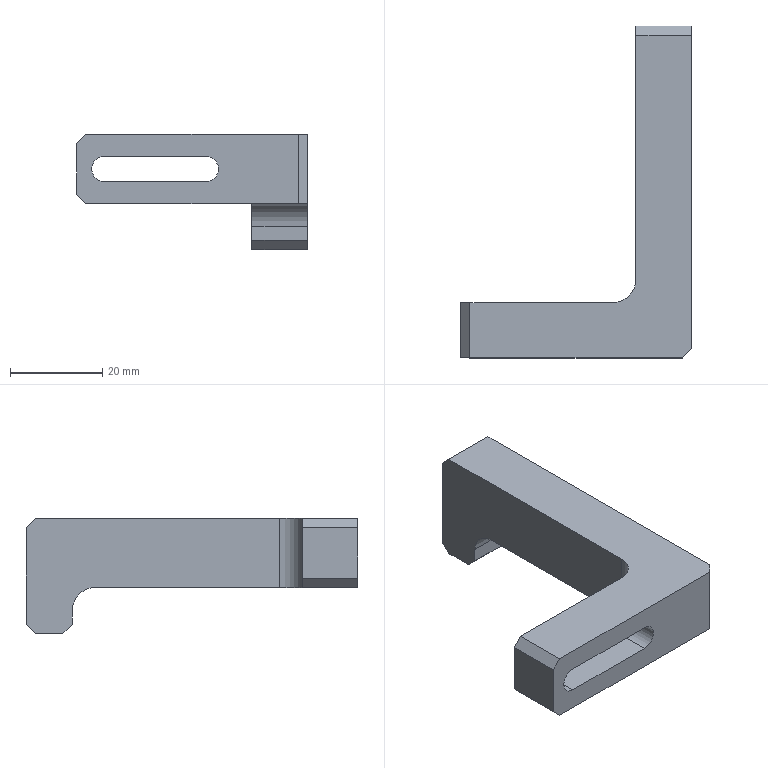NC program | NX | posted with a generic post | part box 50 x 72 x 25 mm
Lines 1 to 975 of 3150:
N10 G17 G21 G94 G90
(ZLEVEL_PROFILE_COPY_COPY_1 , TOOL : D3)
N12 T16 M6
N14 G54
N16 G17 G0 G90 X3.75 Y-1.724 B0. C0. S9500 M3
N18 G43 Z30. H16
N20 Z0.6
N22 G94 G1 Y-3.158 Z0.525 F1000.
N24 X3.81 Y-3.413 Z0.511
N26 X3.95 Y-3.697 Z0.495
N28 X4.25 Y-4.012 Z0.472
N30 X4.639 Y-4.207 Z0.449
N32 X5.071 Y-4.258 Z0.426
N34 X5.495 Y-4.159 Z0.403
N36 X5.86 Y-3.921 Z0.38
N38 X6.062 Y-3.677 Z0.364
N40 X6.185 Y-3.428 Z0.349
N42 X6.25 Y-3.158 Z0.335
N44 Y8. Z-0.25
N46 Y19. F1200.
N48 G3 X5. Y20.25 R1.25
N50 X3.75 Y19. R1.25
N52 G1 Y-3.
N54 G3 X5. Y-4.25 R1.25
N56 X6.25 Y-3. R1.25
N58 G1 Y8.
N60 Y17.625 Z-0.296
N62 X6.246 Y19. Z-0.303
N64 X6.232 Y19.165 Z-0.304
N66 X6.214 Y19.262
N68 X6.174 Y19.415 Z-0.305
N70 X6.132 Y19.513 Z-0.306
N72 X6.048 Y19.665
N74 X5.999 Y19.742 Z-0.307
N76 X5.903 Y19.852 Z-0.308
N78 X5.82 Y19.936
N80 X5.71 Y20.022 Z-0.309
N82 X5.603 Y20.086
N84 X5.44 Y20.161 Z-0.31
N86 X5.339 Y20.197 Z-0.311
N88 X5.186 Y20.227 Z-0.312
N90 X5.056 Y20.241
N92 X4.951 Y20.242 Z-0.313
N94 X4.899
N96 X4.856 Y20.235
N98 X4.77 Y20.221 Z-0.314
N100 X4.586 Y20.17 Z-0.315
N102 X4.495 Y20.14
N104 X4.37 Y20.07 Z-0.316
N106 X4.25 Y19.991
N108 X4.127 Y19.886 Z-0.317
N110 X4.044 Y19.793 Z-0.318
N112 X3.944 Y19.653 Z-0.319
N114 X3.888 Y19.553
N116 X3.843 Y19.454 Z-0.32
N118 X3.821 Y19.404
N120 X3.811 Y19.364
N122 X3.791 Y19.284 Z-0.321
N124 X3.766 Y19.143
N126 X3.754 Y19. Z-0.322
N128 X3.75 Y17.625 Z-0.329
N130 Y-1.625 Z-0.421
N132 X3.754 Y-3. Z-0.428
N134 X3.769 Y-3.18 Z-0.429
N136 X3.79 Y-3.283
N138 X3.843 Y-3.454 Z-0.43
N140 X3.887 Y-3.552 Z-0.431
N142 X3.98 Y-3.71 Z-0.432
N144 X4.057 Y-3.808
N146 X4.185 Y-3.938 Z-0.433
N148 X4.284 Y-4.016 Z-0.434
N150 X4.44 Y-4.11 Z-0.435
N152 X4.556 Y-4.16
N154 X4.73 Y-4.213 Z-0.436
N156 X4.855 Y-4.234 Z-0.437
N158 X5.037 Y-4.242 Z-0.438
N160 X5.163 Y-4.232
N162 X5.341 Y-4.195 Z-0.439
N164 X5.461 Y-4.154 Z-0.44
N166 X5.625 Y-4.074 Z-0.441
N168 X5.731 Y-4.005
N170 X5.868 Y-3.889 Z-0.442
N172 X5.955 Y-3.794 Z-0.443
N174 X6.053 Y-3.659 Z-0.444
N176 X6.112 Y-3.554
N178 X6.155 Y-3.458 Z-0.445
N180 X6.177 Y-3.41
N182 X6.187 Y-3.368
N184 X6.209 Y-3.285 Z-0.446
N186 X6.226 Y-3.214
N188 X6.242 Y-3.144
N190 X6.248 Y-3.072 Z-0.447
N192 X6.25 Y-3.
N194 Y8. Z-0.5
N196 Y17.625 Z-0.546
N198 X6.246 Y19. Z-0.553
N200 X6.232 Y19.165 Z-0.554
N202 X6.214 Y19.262
N204 X6.174 Y19.415 Z-0.555
N206 X6.132 Y19.513 Z-0.556
N208 X6.048 Y19.665
N210 X5.999 Y19.742 Z-0.557
N212 X5.903 Y19.852 Z-0.558
N214 X5.82 Y19.936
N216 X5.71 Y20.022 Z-0.559
N218 X5.603 Y20.086
N220 X5.44 Y20.161 Z-0.56
N222 X5.339 Y20.197 Z-0.561
N224 X5.187 Y20.227 Z-0.562
N226 X5.056 Y20.241
N228 X4.951 Y20.242 Z-0.563
N230 X4.899
N232 X4.856 Y20.235
N234 X4.77 Y20.221 Z-0.564
N236 X4.586 Y20.17 Z-0.565
N238 X4.495 Y20.14
N240 X4.37 Y20.07 Z-0.566
N242 X4.25 Y19.991
N244 X4.127 Y19.886 Z-0.567
N246 X4.044 Y19.793 Z-0.568
N248 X3.944 Y19.653 Z-0.569
N250 X3.888 Y19.553
N252 X3.843 Y19.454 Z-0.57
N254 X3.821 Y19.404
N256 X3.811 Y19.364
N258 X3.791 Y19.284 Z-0.571
N260 X3.766 Y19.143
N262 X3.754 Y19. Z-0.572
N264 X3.75 Y17.625 Z-0.579
N266 Y-1.625 Z-0.671
N268 X3.754 Y-3. Z-0.678
N270 X3.769 Y-3.18 Z-0.679
N272 X3.79 Y-3.283
N274 X3.843 Y-3.454 Z-0.68
N276 X3.887 Y-3.552 Z-0.681
N278 X3.98 Y-3.71 Z-0.682
N280 X4.057 Y-3.808
N282 X4.185 Y-3.938 Z-0.683
N284 X4.284 Y-4.016 Z-0.684
N286 X4.44 Y-4.11 Z-0.685
N288 X4.556 Y-4.16
N290 X4.73 Y-4.213 Z-0.686
N292 X4.855 Y-4.234 Z-0.687
N294 X5.037 Y-4.242 Z-0.688
N296 X5.163 Y-4.232
N298 X5.341 Y-4.195 Z-0.689
N300 X5.461 Y-4.154 Z-0.69
N302 X5.625 Y-4.074 Z-0.691
N304 X5.731 Y-4.005
N306 X5.868 Y-3.889 Z-0.692
N308 X5.955 Y-3.794 Z-0.693
N310 X6.053 Y-3.659 Z-0.694
N312 X6.112 Y-3.554
N314 X6.155 Y-3.458 Z-0.695
N316 X6.177 Y-3.41
N318 X6.187 Y-3.368
N320 X6.209 Y-3.285 Z-0.696
N322 X6.226 Y-3.214
N324 X6.242 Y-3.144
N326 X6.248 Y-3.072 Z-0.697
N328 X6.25 Y-3.
N330 Y8. Z-0.75
N332 Y17.625 Z-0.796
N334 X6.246 Y19. Z-0.803
N336 X6.232 Y19.165 Z-0.804
N338 X6.214 Y19.262
N340 X6.174 Y19.415 Z-0.805
N342 X6.132 Y19.513 Z-0.806
N344 X6.048 Y19.665
N346 X5.999 Y19.742 Z-0.807
N348 X5.903 Y19.852 Z-0.808
N350 X5.82 Y19.936
N352 X5.71 Y20.022 Z-0.809
N354 X5.603 Y20.086
N356 X5.44 Y20.161 Z-0.81
N358 X5.339 Y20.197 Z-0.811
N360 X5.187 Y20.227 Z-0.812
N362 X5.056 Y20.241
N364 X4.951 Y20.242 Z-0.813
N366 X4.899
N368 X4.856 Y20.235
N370 X4.77 Y20.221 Z-0.814
N372 X4.586 Y20.17 Z-0.815
N374 X4.495 Y20.14
N376 X4.37 Y20.07 Z-0.816
N378 X4.25 Y19.991
N380 X4.127 Y19.886 Z-0.817
N382 X4.044 Y19.793 Z-0.818
N384 X3.944 Y19.653 Z-0.819
N386 X3.888 Y19.553
N388 X3.843 Y19.454 Z-0.82
N390 X3.821 Y19.404
N392 X3.811 Y19.364
N394 X3.791 Y19.284 Z-0.821
N396 X3.766 Y19.143
N398 X3.754 Y19. Z-0.822
N400 X3.75 Y17.625 Z-0.829
N402 Y-1.625 Z-0.921
N404 X3.754 Y-3. Z-0.928
N406 X3.769 Y-3.18 Z-0.929
N408 X3.79 Y-3.283
N410 X3.843 Y-3.454 Z-0.93
N412 X3.887 Y-3.552 Z-0.931
N414 X3.98 Y-3.71 Z-0.932
N416 X4.057 Y-3.808
N418 X4.185 Y-3.938 Z-0.933
N420 X4.284 Y-4.016 Z-0.934
N422 X4.44 Y-4.11 Z-0.935
N424 X4.556 Y-4.16
N426 X4.73 Y-4.213 Z-0.936
N428 X4.855 Y-4.234 Z-0.937
N430 X5.037 Y-4.242 Z-0.938
N432 X5.163 Y-4.232
N434 X5.341 Y-4.195 Z-0.939
N436 X5.461 Y-4.154 Z-0.94
N438 X5.625 Y-4.074 Z-0.941
N440 X5.731 Y-4.005
N442 X5.868 Y-3.889 Z-0.942
N444 X5.955 Y-3.794 Z-0.943
N446 X6.053 Y-3.659 Z-0.944
N448 X6.112 Y-3.554
N450 X6.155 Y-3.458 Z-0.945
N452 X6.177 Y-3.41
N454 X6.187 Y-3.368
N456 X6.209 Y-3.285 Z-0.946
N458 X6.226 Y-3.214
N460 X6.242 Y-3.144
N462 X6.248 Y-3.072 Z-0.947
N464 X6.25 Y-3.
N466 Y8. Z-1.
N468 Y17.625 Z-1.046
N470 X6.246 Y19. Z-1.053
N472 X6.232 Y19.165 Z-1.054
N474 X6.214 Y19.262
N476 X6.174 Y19.415 Z-1.055
N478 X6.132 Y19.513 Z-1.056
N480 X6.048 Y19.665
N482 X5.999 Y19.742 Z-1.057
N484 X5.903 Y19.852 Z-1.058
N486 X5.82 Y19.936
N488 X5.71 Y20.022 Z-1.059
N490 X5.603 Y20.086
N492 X5.44 Y20.161 Z-1.06
N494 X5.339 Y20.197 Z-1.061
N496 X5.187 Y20.227 Z-1.062
N498 X5.056 Y20.241
N500 X4.951 Y20.242 Z-1.063
N502 X4.899
N504 X4.856 Y20.235
N506 X4.77 Y20.221 Z-1.064
N508 X4.586 Y20.17 Z-1.065
N510 X4.495 Y20.14
N512 X4.37 Y20.07 Z-1.066
N514 X4.25 Y19.991
N516 X4.127 Y19.886 Z-1.067
N518 X4.044 Y19.793 Z-1.068
N520 X3.944 Y19.653 Z-1.069
N522 X3.888 Y19.553
N524 X3.843 Y19.454 Z-1.07
N526 X3.821 Y19.404
N528 X3.811 Y19.364
N530 X3.791 Y19.284 Z-1.071
N532 X3.766 Y19.143
N534 X3.754 Y19. Z-1.072
N536 X3.75 Y17.625 Z-1.079
N538 Y-1.625 Z-1.171
N540 X3.754 Y-3. Z-1.178
N542 X3.769 Y-3.18 Z-1.179
N544 X3.79 Y-3.283
N546 X3.843 Y-3.454 Z-1.18
N548 X3.887 Y-3.552 Z-1.181
N550 X3.98 Y-3.71 Z-1.182
N552 X4.057 Y-3.808
N554 X4.185 Y-3.938 Z-1.183
N556 X4.284 Y-4.016 Z-1.184
N558 X4.44 Y-4.11 Z-1.185
N560 X4.556 Y-4.16
N562 X4.73 Y-4.213 Z-1.186
N564 X4.855 Y-4.234 Z-1.187
N566 X5.037 Y-4.242 Z-1.188
N568 X5.163 Y-4.232
N570 X5.341 Y-4.195 Z-1.189
N572 X5.461 Y-4.154 Z-1.19
N574 X5.625 Y-4.074 Z-1.191
N576 X5.731 Y-4.005
N578 X5.868 Y-3.889 Z-1.192
N580 X5.955 Y-3.794 Z-1.193
N582 X6.053 Y-3.659 Z-1.194
N584 X6.112 Y-3.554
N586 X6.155 Y-3.458 Z-1.195
N588 X6.176 Y-3.41
N590 X6.187 Y-3.368
N592 X6.209 Y-3.285 Z-1.196
N594 X6.226 Y-3.214
N596 X6.242 Y-3.144
N598 X6.248 Y-3.072 Z-1.197
N600 X6.25 Y-3.
N602 Y8. Z-1.25
N604 Y17.625 Z-1.296
N606 X6.246 Y19. Z-1.303
N608 X6.232 Y19.165 Z-1.304
N610 X6.214 Y19.262
N612 X6.174 Y19.415 Z-1.305
N614 X6.131 Y19.513 Z-1.306
N616 X6.048 Y19.665
N618 X5.999 Y19.742 Z-1.307
N620 X5.903 Y19.852 Z-1.308
N622 X5.82 Y19.936
N624 X5.71 Y20.022 Z-1.309
N626 X5.603 Y20.086
N628 X5.44 Y20.161 Z-1.31
N630 X5.339 Y20.197 Z-1.311
N632 X5.187 Y20.227 Z-1.312
N634 X5.056 Y20.241
N636 X4.951 Z-1.313
N638 X4.899 Y20.242
N640 X4.856 Y20.235
N642 X4.77 Y20.221 Z-1.314
N644 X4.586 Y20.17 Z-1.315
N646 X4.495 Y20.14
N648 X4.37 Y20.07 Z-1.316
N650 X4.25 Y19.991
N652 X4.127 Y19.886 Z-1.317
N654 X4.044 Y19.793 Z-1.318
N656 X3.944 Y19.653 Z-1.319
N658 X3.888 Y19.553
N660 X3.843 Y19.454 Z-1.32
N662 X3.821 Y19.404
N664 X3.811 Y19.364
N666 X3.791 Y19.284 Z-1.321
N668 X3.766 Y19.143
N670 X3.754 Y19. Z-1.322
N672 X3.75 Y17.625 Z-1.329
N674 Y-1.625 Z-1.421
N676 X3.754 Y-3. Z-1.428
N678 X3.769 Y-3.18 Z-1.429
N680 X3.79 Y-3.283
N682 X3.843 Y-3.454 Z-1.43
N684 X3.887 Y-3.552 Z-1.431
N686 X3.98 Y-3.71 Z-1.432
N688 X4.057 Y-3.808
N690 X4.185 Y-3.938 Z-1.433
N692 X4.284 Y-4.016 Z-1.434
N694 X4.44 Y-4.11 Z-1.435
N696 X4.556 Y-4.16
N698 X4.73 Y-4.213 Z-1.436
N700 X4.855 Y-4.234 Z-1.437
N702 X5.037 Y-4.242 Z-1.438
N704 X5.163 Y-4.232
N706 X5.341 Y-4.195 Z-1.439
N708 X5.461 Y-4.154 Z-1.44
N710 X5.625 Y-4.074 Z-1.441
N712 X5.731 Y-4.005
N714 X5.868 Y-3.889 Z-1.442
N716 X5.955 Y-3.794 Z-1.443
N718 X6.053 Y-3.659 Z-1.444
N720 X6.112 Y-3.554
N722 X6.155 Y-3.458 Z-1.445
N724 X6.176 Y-3.41
N726 X6.187 Y-3.368
N728 X6.209 Y-3.285 Z-1.446
N730 X6.226 Y-3.214
N732 X6.242 Y-3.144
N734 X6.248 Y-3.072 Z-1.447
N736 X6.25 Y-3.
N738 Y8. Z-1.5
N740 Y17.625 Z-1.546
N742 X6.246 Y19. Z-1.553
N744 X6.232 Y19.165 Z-1.554
N746 X6.214 Y19.262
N748 X6.174 Y19.415 Z-1.555
N750 X6.131 Y19.513 Z-1.556
N752 X6.048 Y19.665
N754 X5.999 Y19.742 Z-1.557
N756 X5.903 Y19.852 Z-1.558
N758 X5.82 Y19.936
N760 X5.71 Y20.022 Z-1.559
N762 X5.603 Y20.086
N764 X5.44 Y20.161 Z-1.56
N766 X5.339 Y20.197 Z-1.561
N768 X5.187 Y20.227 Z-1.562
N770 X5.056 Y20.241
N772 X4.951 Z-1.563
N774 X4.899 Y20.242
N776 X4.856 Y20.235
N778 X4.77 Y20.221 Z-1.564
N780 X4.586 Y20.17 Z-1.565
N782 X4.495 Y20.14
N784 X4.37 Y20.07 Z-1.566
N786 X4.25 Y19.991
N788 X4.127 Y19.886 Z-1.567
N790 X4.044 Y19.793 Z-1.568
N792 X3.944 Y19.653 Z-1.569
N794 X3.888 Y19.553
N796 X3.843 Y19.454 Z-1.57
N798 X3.821 Y19.404
N800 X3.811 Y19.364
N802 X3.791 Y19.284 Z-1.571
N804 X3.766 Y19.143
N806 X3.754 Y19. Z-1.572
N808 X3.75 Y17.625 Z-1.579
N810 Y-1.625 Z-1.671
N812 X3.754 Y-3. Z-1.678
N814 X3.769 Y-3.18 Z-1.679
N816 X3.79 Y-3.283
N818 X3.843 Y-3.454 Z-1.68
N820 X3.887 Y-3.552 Z-1.681
N822 X3.98 Y-3.71 Z-1.682
N824 X4.057 Y-3.808
N826 X4.185 Y-3.938 Z-1.683
N828 X4.284 Y-4.016 Z-1.684
N830 X4.44 Y-4.11 Z-1.685
N832 X4.556 Y-4.16
N834 X4.73 Y-4.213 Z-1.686
N836 X4.855 Y-4.234 Z-1.687
N838 X5.037 Y-4.242 Z-1.688
N840 X5.163 Y-4.232
N842 X5.341 Y-4.195 Z-1.689
N844 X5.461 Y-4.154 Z-1.69
N846 X5.625 Y-4.074 Z-1.691
N848 X5.731 Y-4.005
N850 X5.868 Y-3.889 Z-1.692
N852 X5.955 Y-3.794 Z-1.693
N854 X6.053 Y-3.659 Z-1.694
N856 X6.112 Y-3.554
N858 X6.155 Y-3.458 Z-1.695
N860 X6.176 Y-3.41
N862 X6.187 Y-3.368
N864 X6.209 Y-3.285 Z-1.696
N866 X6.226 Y-3.214
N868 X6.242 Y-3.144
N870 X6.248 Y-3.072 Z-1.697
N872 X6.25 Y-3.
N874 Y8. Z-1.75
N876 Y17.625 Z-1.796
N878 X6.246 Y19. Z-1.803
N880 X6.232 Y19.165 Z-1.804
N882 X6.214 Y19.262
N884 X6.174 Y19.415 Z-1.805
N886 X6.131 Y19.513 Z-1.806
N888 X6.048 Y19.665
N890 X5.999 Y19.742 Z-1.807
N892 X5.903 Y19.852 Z-1.808
N894 X5.82 Y19.936
N896 X5.71 Y20.022 Z-1.809
N898 X5.603 Y20.086
N900 X5.44 Y20.161 Z-1.81
N902 X5.339 Y20.197 Z-1.811
N904 X5.187 Y20.227 Z-1.812
N906 X5.056 Y20.241
N908 X4.951 Z-1.813
N910 X4.899 Y20.242
N912 X4.856 Y20.235
N914 X4.77 Y20.221 Z-1.814
N916 X4.586 Y20.17 Z-1.815
N918 X4.495 Y20.14
N920 X4.37 Y20.07 Z-1.816
N922 X4.25 Y19.991
N924 X4.127 Y19.886 Z-1.817
N926 X4.044 Y19.793 Z-1.818
N928 X3.944 Y19.653 Z-1.819
N930 X3.888 Y19.553
N932 X3.843 Y19.454 Z-1.82
N934 X3.821 Y19.404
N936 X3.811 Y19.364
N938 X3.791 Y19.284 Z-1.821
N940 X3.766 Y19.143
N942 X3.754 Y19. Z-1.822
N944 X3.75 Y17.625 Z-1.829
N946 Y-1.625 Z-1.921
N948 X3.754 Y-3. Z-1.928
N950 X3.769 Y-3.18 Z-1.929
N952 X3.79 Y-3.283
N954 X3.843 Y-3.454 Z-1.93
N956 X3.887 Y-3.552 Z-1.931
N958 X3.98 Y-3.71 Z-1.932
N960 X4.057 Y-3.808
N962 X4.185 Y-3.938 Z-1.933
N964 X4.284 Y-4.016 Z-1.934
N966 X4.44 Y-4.11 Z-1.935
N968 X4.556 Y-4.16
N970 X4.73 Y-4.213 Z-1.936
N972 X4.855 Y-4.234 Z-1.937
N974 X5.037 Y-4.242 Z-1.938
N976 X5.163 Y-4.232
N978 X5.341 Y-4.195 Z-1.939
N980 X5.461 Y-4.154 Z-1.94
N982 X5.625 Y-4.074 Z-1.941
N984 X5.731 Y-4.005
N986 X5.868 Y-3.889 Z-1.942
N988 X5.955 Y-3.794 Z-1.943
N990 X6.053 Y-3.659 Z-1.944
N992 X6.112 Y-3.554
N994 X6.155 Y-3.458 Z-1.945
N996 X6.176 Y-3.41
N998 X6.187 Y-3.368
N1000 X6.209 Y-3.285 Z-1.946
N1002 X6.226 Y-3.214
N1004 X6.242 Y-3.144
N1006 X6.248 Y-3.072 Z-1.947
N1008 X6.25 Y-3.
N1010 Y8. Z-2.
N1012 Y17.625 Z-2.046
N1014 X6.246 Y19. Z-2.053
N1016 X6.232 Y19.165 Z-2.054
N1018 X6.214 Y19.262
N1020 X6.174 Y19.415 Z-2.055
N1022 X6.131 Y19.513 Z-2.056
N1024 X6.048 Y19.665
N1026 X5.999 Y19.742 Z-2.057
N1028 X5.903 Y19.852 Z-2.058
N1030 X5.82 Y19.936
N1032 X5.71 Y20.022 Z-2.059
N1034 X5.603 Y20.086
N1036 X5.44 Y20.161 Z-2.06
N1038 X5.339 Y20.197 Z-2.061
N1040 X5.187 Y20.227 Z-2.062
N1042 X5.056 Y20.241
N1044 X4.951 Z-2.063
N1046 X4.899 Y20.242
N1048 X4.856 Y20.235
N1050 X4.77 Y20.221 Z-2.064
N1052 X4.586 Y20.17 Z-2.065
N1054 X4.495 Y20.14
N1056 X4.37 Y20.07 Z-2.066
N1058 X4.25 Y19.991
N1060 X4.127 Y19.886 Z-2.067
N1062 X4.044 Y19.793 Z-2.068
N1064 X3.944 Y19.653 Z-2.069
N1066 X3.888 Y19.553
N1068 X3.843 Y19.454 Z-2.07
N1070 X3.821 Y19.404
N1072 X3.811 Y19.364
N1074 X3.791 Y19.284 Z-2.071
N1076 X3.766 Y19.143
N1078 X3.754 Y19. Z-2.072
N1080 X3.75 Y17.625 Z-2.079
N1082 Y-1.625 Z-2.171
N1084 X3.754 Y-3. Z-2.178
N1086 X3.769 Y-3.18 Z-2.179
N1088 X3.79 Y-3.283
N1090 X3.843 Y-3.454 Z-2.18
N1092 X3.887 Y-3.552 Z-2.181
N1094 X3.98 Y-3.71 Z-2.182
N1096 X4.057 Y-3.808
N1098 X4.185 Y-3.938 Z-2.183
N1100 X4.284 Y-4.016 Z-2.184
N1102 X4.44 Y-4.11 Z-2.185
N1104 X4.556 Y-4.16
N1106 X4.73 Y-4.213 Z-2.186
N1108 X4.855 Y-4.234 Z-2.187
N1110 X5.037 Y-4.242 Z-2.188
N1112 X5.163 Y-4.232
N1114 X5.341 Y-4.195 Z-2.189
N1116 X5.461 Y-4.154 Z-2.19
N1118 X5.625 Y-4.074 Z-2.191
N1120 X5.731 Y-4.005
N1122 X5.868 Y-3.889 Z-2.192
N1124 X5.955 Y-3.794 Z-2.193
N1126 X6.053 Y-3.659 Z-2.194
N1128 X6.112 Y-3.554
N1130 X6.155 Y-3.458 Z-2.195
N1132 X6.176 Y-3.41
N1134 X6.187 Y-3.368
N1136 X6.209 Y-3.285 Z-2.196
N1138 X6.226 Y-3.214
N1140 X6.242 Y-3.144
N1142 X6.248 Y-3.072 Z-2.197
N1144 X6.25 Y-3.
N1146 Y8. Z-2.25
N1148 Y17.625 Z-2.296
N1150 X6.246 Y19. Z-2.303
N1152 X6.232 Y19.165 Z-2.304
N1154 X6.214 Y19.262
N1156 X6.174 Y19.415 Z-2.305
N1158 X6.131 Y19.513 Z-2.306
N1160 X6.048 Y19.665
N1162 X5.999 Y19.742 Z-2.307
N1164 X5.903 Y19.852 Z-2.308
N1166 X5.82 Y19.936
N1168 X5.71 Y20.022 Z-2.309
N1170 X5.603 Y20.086
N1172 X5.44 Y20.161 Z-2.31
N1174 X5.339 Y20.197 Z-2.311
N1176 X5.187 Y20.227 Z-2.312
N1178 X5.056 Y20.241
N1180 X4.951 Z-2.313
N1182 X4.899 Y20.242
N1184 X4.856 Y20.235
N1186 X4.77 Y20.221 Z-2.314
N1188 X4.586 Y20.17 Z-2.315
N1190 X4.495 Y20.14
N1192 X4.37 Y20.07 Z-2.316
N1194 X4.251 Y19.991
N1196 X4.127 Y19.886 Z-2.317
N1198 X4.044 Y19.793 Z-2.318
N1200 X3.944 Y19.653 Z-2.319
N1202 X3.888 Y19.553
N1204 X3.843 Y19.454 Z-2.32
N1206 X3.821 Y19.404
N1208 X3.811 Y19.364
N1210 X3.791 Y19.284 Z-2.321
N1212 X3.766 Y19.143
N1214 X3.754 Y19. Z-2.322
N1216 X3.75 Y17.625 Z-2.329
N1218 Y-1.625 Z-2.421
N1220 X3.754 Y-3. Z-2.428
N1222 X3.769 Y-3.18 Z-2.429
N1224 X3.79 Y-3.283
N1226 X3.843 Y-3.454 Z-2.43
N1228 X3.887 Y-3.552 Z-2.431
N1230 X3.98 Y-3.71 Z-2.432
N1232 X4.057 Y-3.808
N1234 X4.185 Y-3.938 Z-2.433
N1236 X4.284 Y-4.016 Z-2.434
N1238 X4.44 Y-4.11 Z-2.435
N1240 X4.556 Y-4.16
N1242 X4.73 Y-4.213 Z-2.436
N1244 X4.855 Y-4.234 Z-2.437
N1246 X5.037 Y-4.242 Z-2.438
N1248 X5.163 Y-4.232
N1250 X5.341 Y-4.195 Z-2.439
N1252 X5.461 Y-4.154 Z-2.44
N1254 X5.625 Y-4.074 Z-2.441
N1256 X5.731 Y-4.005
N1258 X5.868 Y-3.889 Z-2.442
N1260 X5.955 Y-3.794 Z-2.443
N1262 X6.053 Y-3.659 Z-2.444
N1264 X6.112 Y-3.554
N1266 X6.155 Y-3.458 Z-2.445
N1268 X6.176 Y-3.41
N1270 X6.187 Y-3.368
N1272 X6.209 Y-3.285 Z-2.446
N1274 X6.226 Y-3.214
N1276 X6.242 Y-3.144
N1278 X6.248 Y-3.072 Z-2.447
N1280 X6.25 Y-3.
N1282 Y8. Z-2.5
N1284 Y17.625 Z-2.546
N1286 X6.246 Y19. Z-2.553
N1288 X6.232 Y19.165 Z-2.554
N1290 X6.214 Y19.262
N1292 X6.174 Y19.415 Z-2.555
N1294 X6.131 Y19.513 Z-2.556
N1296 X6.048 Y19.665
N1298 X5.999 Y19.742 Z-2.557
N1300 X5.903 Y19.852 Z-2.558
N1302 X5.82 Y19.936
N1304 X5.71 Y20.022 Z-2.559
N1306 X5.603 Y20.086
N1308 X5.44 Y20.161 Z-2.56
N1310 X5.339 Y20.197 Z-2.561
N1312 X5.187 Y20.227 Z-2.562
N1314 X5.056 Y20.241
N1316 X4.951 Z-2.563
N1318 X4.899 Y20.242
N1320 X4.856 Y20.235
N1322 X4.77 Y20.221 Z-2.564
N1324 X4.586 Y20.17 Z-2.565
N1326 X4.495 Y20.14
N1328 X4.37 Y20.07 Z-2.566
N1330 X4.251 Y19.991
N1332 X4.127 Y19.886 Z-2.567
N1334 X4.044 Y19.793 Z-2.568
N1336 X3.944 Y19.653 Z-2.569
N1338 X3.888 Y19.553
N1340 X3.843 Y19.454 Z-2.57
N1342 X3.821 Y19.404
N1344 X3.811 Y19.364
N1346 X3.791 Y19.284 Z-2.571
N1348 X3.766 Y19.143
N1350 X3.754 Y19. Z-2.572
N1352 X3.75 Y17.625 Z-2.579
N1354 Y-1.625 Z-2.671
N1356 X3.754 Y-3. Z-2.678
N1358 X3.769 Y-3.18 Z-2.679
N1360 X3.79 Y-3.283
N1362 X3.843 Y-3.454 Z-2.68
N1364 X3.887 Y-3.552 Z-2.681
N1366 X3.98 Y-3.71 Z-2.682
N1368 X4.057 Y-3.808
N1370 X4.185 Y-3.938 Z-2.683
N1372 X4.284 Y-4.016 Z-2.684
N1374 X4.44 Y-4.11 Z-2.685
N1376 X4.556 Y-4.16
N1378 X4.73 Y-4.213 Z-2.686
N1380 X4.855 Y-4.234 Z-2.687
N1382 X5.037 Y-4.242 Z-2.688
N1384 X5.163 Y-4.232
N1386 X5.341 Y-4.195 Z-2.689
N1388 X5.461 Y-4.154 Z-2.69
N1390 X5.625 Y-4.074 Z-2.691
N1392 X5.731 Y-4.005
N1394 X5.868 Y-3.889 Z-2.692
N1396 X5.955 Y-3.794 Z-2.693
N1398 X6.053 Y-3.659 Z-2.694
N1400 X6.112 Y-3.554
N1402 X6.155 Y-3.458 Z-2.695
N1404 X6.176 Y-3.41
N1406 X6.187 Y-3.368
N1408 X6.209 Y-3.285 Z-2.696
N1410 X6.226 Y-3.214
N1412 X6.242 Y-3.144
N1414 X6.248 Y-3.072 Z-2.697
N1416 X6.25 Y-3.
N1418 Y8. Z-2.75
N1420 Y17.625 Z-2.796
N1422 X6.246 Y19. Z-2.803
N1424 X6.232 Y19.165 Z-2.804
N1426 X6.214 Y19.262
N1428 X6.174 Y19.415 Z-2.805
N1430 X6.131 Y19.513 Z-2.806
N1432 X6.048 Y19.665
N1434 X5.999 Y19.742 Z-2.807
N1436 X5.903 Y19.852 Z-2.808
N1438 X5.82 Y19.936
N1440 X5.71 Y20.022 Z-2.809
N1442 X5.603 Y20.086
N1444 X5.44 Y20.161 Z-2.81
N1446 X5.339 Y20.197 Z-2.811
N1448 X5.187 Y20.227 Z-2.812
N1450 X5.056 Y20.241
N1452 X4.951 Z-2.813
N1454 X4.899 Y20.242
N1456 X4.856 Y20.235
N1458 X4.77 Y20.221 Z-2.814
N1460 X4.586 Y20.17 Z-2.815
N1462 X4.495 Y20.14
N1464 X4.37 Y20.07 Z-2.816
N1466 X4.251 Y19.991
N1468 X4.127 Y19.886 Z-2.817
N1470 X4.044 Y19.793 Z-2.818
N1472 X3.944 Y19.653 Z-2.819
N1474 X3.888 Y19.553
N1476 X3.843 Y19.454 Z-2.82
N1478 X3.821 Y19.404
N1480 X3.811 Y19.364
N1482 X3.791 Y19.284 Z-2.821
N1484 X3.766 Y19.143
N1486 X3.754 Y19. Z-2.822
N1488 X3.75 Y17.625 Z-2.829
N1490 Y-1.625 Z-2.921
N1492 X3.754 Y-3. Z-2.928
N1494 X3.769 Y-3.18 Z-2.929
N1496 X3.79 Y-3.283
N1498 X3.843 Y-3.454 Z-2.93
N1500 X3.887 Y-3.552 Z-2.931
N1502 X3.98 Y-3.71 Z-2.932
N1504 X4.057 Y-3.808
N1506 X4.185 Y-3.938 Z-2.933
N1508 X4.284 Y-4.016 Z-2.934
N1510 X4.44 Y-4.11 Z-2.935
N1512 X4.556 Y-4.16
N1514 X4.73 Y-4.213 Z-2.936
N1516 X4.855 Y-4.234 Z-2.937
N1518 X5.037 Y-4.242 Z-2.938
N1520 X5.163 Y-4.232
N1522 X5.341 Y-4.195 Z-2.939
N1524 X5.461 Y-4.154 Z-2.94
N1526 X5.625 Y-4.074 Z-2.941
N1528 X5.731 Y-4.005
N1530 X5.868 Y-3.889 Z-2.942
N1532 X5.955 Y-3.794 Z-2.943
N1534 X6.053 Y-3.659 Z-2.944
N1536 X6.112 Y-3.554
N1538 X6.155 Y-3.458 Z-2.945
N1540 X6.176 Y-3.41
N1542 X6.187 Y-3.368
N1544 X6.209 Y-3.285 Z-2.946
N1546 X6.226 Y-3.214
N1548 X6.242 Y-3.144
N1550 X6.248 Y-3.072 Z-2.947
N1552 X6.25 Y-3.
N1554 Y8. Z-3.
N1556 Y17.625 Z-3.046
N1558 X6.246 Y19. Z-3.053
N1560 X6.232 Y19.165 Z-3.054
N1562 X6.214 Y19.262
N1564 X6.174 Y19.415 Z-3.055
N1566 X6.131 Y19.513 Z-3.056
N1568 X6.048 Y19.665
N1570 X5.999 Y19.742 Z-3.057
N1572 X5.903 Y19.852 Z-3.058
N1574 X5.82 Y19.936
N1576 X5.71 Y20.022 Z-3.059
N1578 X5.603 Y20.086
N1580 X5.44 Y20.161 Z-3.06
N1582 X5.339 Y20.197 Z-3.061
N1584 X5.187 Y20.227 Z-3.062
N1586 X5.056 Y20.241
N1588 X4.951 Z-3.063
N1590 X4.899 Y20.242
N1592 X4.856 Y20.235
N1594 X4.77 Y20.221 Z-3.064
N1596 X4.586 Y20.17 Z-3.065
N1598 X4.495 Y20.14
N1600 X4.37 Y20.07 Z-3.066
N1602 X4.251 Y19.991
N1604 X4.127 Y19.886 Z-3.067
N1606 X4.044 Y19.793 Z-3.068
N1608 X3.944 Y19.653 Z-3.069
N1610 X3.888 Y19.553
N1612 X3.843 Y19.454 Z-3.07
N1614 X3.821 Y19.404
N1616 X3.811 Y19.364
N1618 X3.791 Y19.284 Z-3.071
N1620 X3.766 Y19.143
N1622 X3.754 Y19. Z-3.072
N1624 X3.75 Y17.625 Z-3.079
N1626 Y-1.625 Z-3.171
N1628 X3.754 Y-3. Z-3.178
N1630 X3.769 Y-3.18 Z-3.179
N1632 X3.79 Y-3.283
N1634 X3.843 Y-3.454 Z-3.18
N1636 X3.887 Y-3.552 Z-3.181
N1638 X3.98 Y-3.71 Z-3.182
N1640 X4.057 Y-3.808
N1642 X4.185 Y-3.938 Z-3.183
N1644 X4.284 Y-4.016 Z-3.184
N1646 X4.44 Y-4.11 Z-3.185
N1648 X4.556 Y-4.16
N1650 X4.73 Y-4.213 Z-3.186
N1652 X4.855 Y-4.234 Z-3.187
N1654 X5.037 Y-4.242 Z-3.188
N1656 X5.163 Y-4.232
N1658 X5.341 Y-4.195 Z-3.189
N1660 X5.461 Y-4.154 Z-3.19
N1662 X5.625 Y-4.074 Z-3.191
N1664 X5.731 Y-4.005
N1666 X5.868 Y-3.889 Z-3.192
N1668 X5.955 Y-3.794 Z-3.193
N1670 X6.053 Y-3.659 Z-3.194
N1672 X6.112 Y-3.554
N1674 X6.155 Y-3.458 Z-3.195
N1676 X6.176 Y-3.41
N1678 X6.187 Y-3.368
N1680 X6.209 Y-3.285 Z-3.196
N1682 X6.226 Y-3.214
N1684 X6.242 Y-3.144
N1686 X6.248 Y-3.072 Z-3.197
N1688 X6.25 Y-3.
N1690 Y8. Z-3.25
N1692 Y17.625 Z-3.296
N1694 X6.246 Y19. Z-3.303
N1696 X6.232 Y19.165 Z-3.304
N1698 X6.214 Y19.262
N1700 X6.174 Y19.415 Z-3.305
N1702 X6.131 Y19.513 Z-3.306
N1704 X6.048 Y19.665
N1706 X5.999 Y19.742 Z-3.307
N1708 X5.903 Y19.852 Z-3.308
N1710 X5.82 Y19.936
N1712 X5.71 Y20.022 Z-3.309
N1714 X5.603 Y20.086
N1716 X5.44 Y20.161 Z-3.31
N1718 X5.339 Y20.197 Z-3.311
N1720 X5.187 Y20.227 Z-3.312
N1722 X5.056 Y20.241
N1724 X4.951 Z-3.313
N1726 X4.899 Y20.242
N1728 X4.856 Y20.235
N1730 X4.77 Y20.221 Z-3.314
N1732 X4.586 Y20.17 Z-3.315
N1734 X4.495 Y20.14
N1736 X4.37 Y20.07 Z-3.316
N1738 X4.251 Y19.991
N1740 X4.127 Y19.886 Z-3.317
N1742 X4.044 Y19.793 Z-3.318
N1744 X3.944 Y19.653 Z-3.319
N1746 X3.888 Y19.553
N1748 X3.843 Y19.454 Z-3.32
N1750 X3.821 Y19.404
N1752 X3.811 Y19.364
N1754 X3.791 Y19.284 Z-3.321
N1756 X3.766 Y19.143
N1758 X3.754 Y19. Z-3.322
N1760 X3.75 Y17.625 Z-3.329
N1762 Y-1.625 Z-3.421
N1764 X3.754 Y-3. Z-3.428
N1766 X3.769 Y-3.18 Z-3.429
N1768 X3.79 Y-3.283
N1770 X3.843 Y-3.454 Z-3.43
N1772 X3.887 Y-3.552 Z-3.431
N1774 X3.98 Y-3.71 Z-3.432
N1776 X4.057 Y-3.808
N1778 X4.185 Y-3.938 Z-3.433
N1780 X4.284 Y-4.016 Z-3.434
N1782 X4.44 Y-4.11 Z-3.435
N1784 X4.556 Y-4.16
N1786 X4.73 Y-4.213 Z-3.436
N1788 X4.855 Y-4.234 Z-3.437
N1790 X5.037 Y-4.242 Z-3.438
N1792 X5.163 Y-4.232
N1794 X5.341 Y-4.195 Z-3.439
N1796 X5.461 Y-4.154 Z-3.44
N1798 X5.625 Y-4.074 Z-3.441
N1800 X5.731 Y-4.005
N1802 X5.868 Y-3.889 Z-3.442
N1804 X5.955 Y-3.794 Z-3.443
N1806 X6.053 Y-3.659 Z-3.444
N1808 X6.112 Y-3.554
N1810 X6.155 Y-3.458 Z-3.445
N1812 X6.176 Y-3.41
N1814 X6.187 Y-3.368
N1816 X6.209 Y-3.285 Z-3.446
N1818 X6.226 Y-3.214
N1820 X6.242 Y-3.144
N1822 X6.248 Y-3.072 Z-3.447
N1824 X6.25 Y-3.
N1826 Y8. Z-3.5
N1828 Y17.625 Z-3.546
N1830 X6.246 Y19. Z-3.553
N1832 X6.232 Y19.165 Z-3.554
N1834 X6.214 Y19.262
N1836 X6.174 Y19.415 Z-3.555
N1838 X6.131 Y19.513 Z-3.556
N1840 X6.048 Y19.665
N1842 X5.999 Y19.742 Z-3.557
N1844 X5.903 Y19.852 Z-3.558
N1846 X5.82 Y19.936
N1848 X5.71 Y20.022 Z-3.559
N1850 X5.603 Y20.086
N1852 X5.44 Y20.161 Z-3.56
N1854 X5.339 Y20.197 Z-3.561
N1856 X5.187 Y20.227 Z-3.562
N1858 X5.056 Y20.241
N1860 X4.951 Z-3.563
N1862 X4.899 Y20.242
N1864 X4.856 Y20.235
N1866 X4.77 Y20.221 Z-3.564
N1868 X4.586 Y20.17 Z-3.565
N1870 X4.495 Y20.14
N1872 X4.37 Y20.07 Z-3.566
N1874 X4.251 Y19.991
N1876 X4.127 Y19.886 Z-3.567
N1878 X4.044 Y19.793 Z-3.568
N1880 X3.944 Y19.653 Z-3.569
N1882 X3.888 Y19.553
N1884 X3.843 Y19.454 Z-3.57
N1886 X3.821 Y19.404
N1888 X3.811 Y19.364
N1890 X3.791 Y19.284 Z-3.571
N1892 X3.766 Y19.143
N1894 X3.754 Y19. Z-3.572
N1896 X3.75 Y17.625 Z-3.579
N1898 Y-1.625 Z-3.671
N1900 X3.754 Y-3. Z-3.678
N1902 X3.769 Y-3.18 Z-3.679
N1904 X3.79 Y-3.283
N1906 X3.843 Y-3.454 Z-3.68
N1908 X3.887 Y-3.552 Z-3.681
N1910 X3.98 Y-3.71 Z-3.682
N1912 X4.057 Y-3.808
N1914 X4.185 Y-3.938 Z-3.683
N1916 X4.284 Y-4.016 Z-3.684
N1918 X4.44 Y-4.11 Z-3.685
N1920 X4.556 Y-4.16
N1922 X4.73 Y-4.213 Z-3.686
N1924 X4.855 Y-4.234 Z-3.687
N1926 X5.037 Y-4.242 Z-3.688
N1928 X5.163 Y-4.232
N1930 X5.341 Y-4.195 Z-3.689
N1932 X5.461 Y-4.154 Z-3.69
N1934 X5.625 Y-4.074 Z-3.691
N1936 X5.731 Y-4.005
N1938 X5.868 Y-3.889 Z-3.692
N1940 X5.955 Y-3.794 Z-3.693
N1942 X6.053 Y-3.659 Z-3.694
N1944 X6.112 Y-3.554
N1946 X6.155 Y-3.458 Z-3.695
N1948 X6.176 Y-3.41